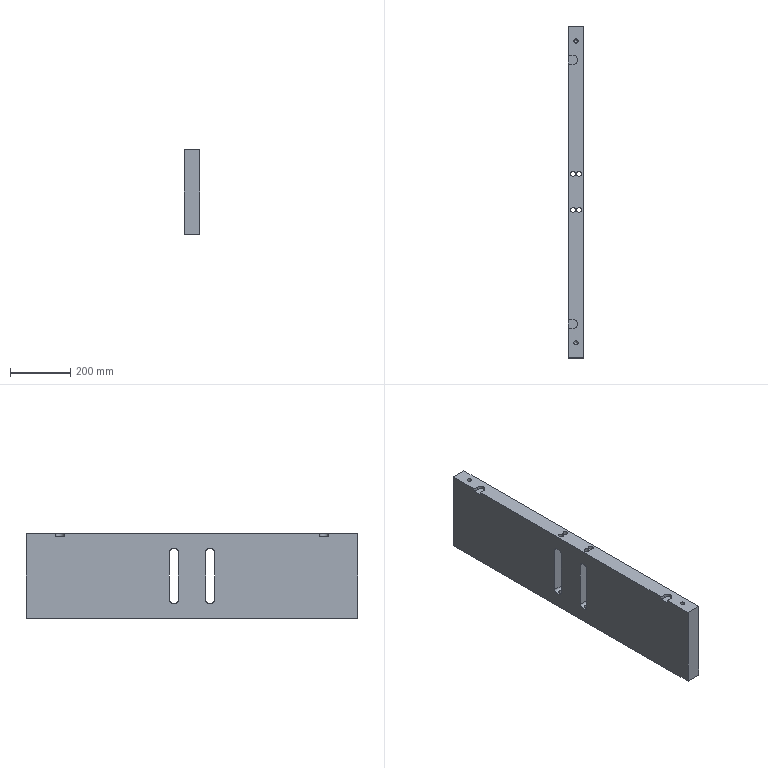Part | NX | features 29 2 | 1 solid | 56 faces | box 50 x 1105 x 280.5 mm | volume 14837944 mm3 | plane 28 | cylinder 23 | cone 5 | commonest cylinder face diameters 16 x8 20 x8 14.1 x5 29 x2